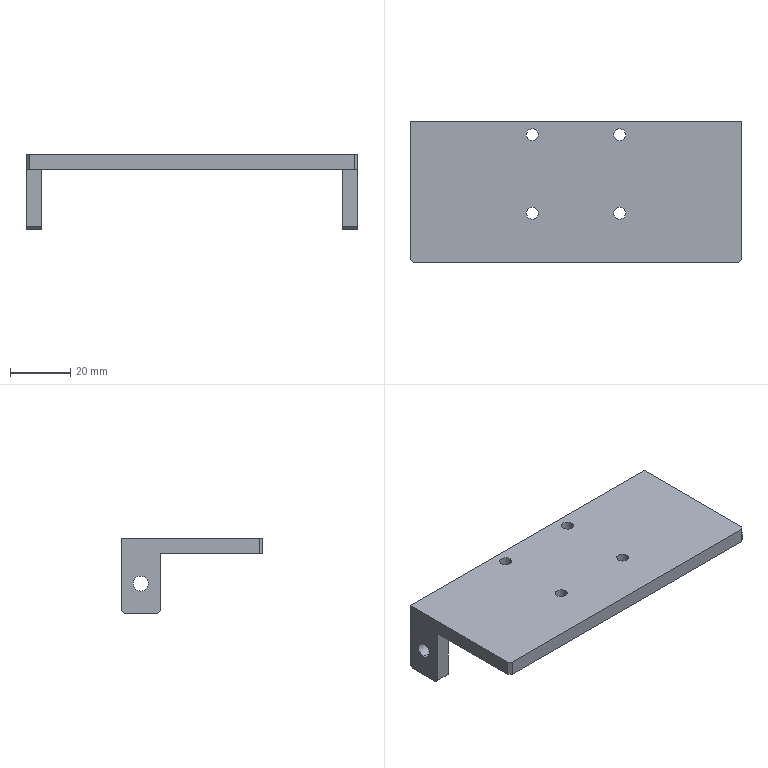Part | STEP file | Guide wheel mechanism revised.sldasm-Part-392 | 1 solid | 30 faces | box 110 x 47 x 25 mm | volume 27987 mm3 | plane 18 | cylinder 12 | commonest cylinder face diameters 4 x8 5 x4
STEP:
#1=CARTESIAN_POINT('',(55.,40.5,-12.5));
#2=VERTEX_POINT('',#1);
#3=CARTESIAN_POINT('',(55.,40.5,-17.5));
#4=VERTEX_POINT('',#3);
#5=CARTESIAN_POINT('',(55.,40.5,-15.));
#6=DIRECTION('',(1.,0.,0.));
#7=DIRECTION('',(0.,0.,1.));
#8=AXIS2_PLACEMENT_3D('',#5,#6,#7);
#9=CIRCLE('',#8,2.5);
#10=EDGE_CURVE('',#2,#4,#9,.T.);
#11=ORIENTED_EDGE('',*,*,#10,.T.);
#12=CARTESIAN_POINT('',(50.,40.5,-17.5));
#13=VERTEX_POINT('',#12);
#14=CARTESIAN_POINT('',(94.446,40.5,-17.5));
#15=DIRECTION('',(-1.,0.,0.));
#16=VECTOR('',#15,1000.);
#17=LINE('',#14,#16);
#18=EDGE_CURVE('',#4,#13,#17,.T.);
#19=ORIENTED_EDGE('',*,*,#18,.T.);
#20=CARTESIAN_POINT('',(50.,40.5,-12.5));
#21=VERTEX_POINT('',#20);
#22=CARTESIAN_POINT('',(50.,40.5,-15.));
#23=DIRECTION('',(-1.,0.,0.));
#24=DIRECTION('',(0.,0.,1.));
#25=AXIS2_PLACEMENT_3D('',#22,#23,#24);
#26=CIRCLE('',#25,2.5);
#27=EDGE_CURVE('',#13,#21,#26,.T.);
#28=ORIENTED_EDGE('',*,*,#27,.T.);
#29=CARTESIAN_POINT('',(94.446,40.5,-12.5));
#30=DIRECTION('',(-1.,0.,0.));
#31=VECTOR('',#30,1000.);
#32=LINE('',#29,#31);
#33=EDGE_CURVE('',#2,#21,#32,.T.);
#34=ORIENTED_EDGE('',*,*,#33,.F.);
#35=EDGE_LOOP('',(#11,#19,#28,#34));
#36=FACE_OUTER_BOUND('',#35,.T.);
#37=CARTESIAN_POINT('',(94.446,40.5,-15.));
#38=DIRECTION('',(-1.,0.,0.));
#39=DIRECTION('',(0.,0.,1.));
#40=AXIS2_PLACEMENT_3D('',#37,#38,#39);
#41=CYLINDRICAL_SURFACE('',#40,2.5);
#42=ADVANCED_FACE('',(#36),#41,.F.);
#43=CARTESIAN_POINT('',(-50.,40.5,-12.5));
#44=VERTEX_POINT('',#43);
#45=CARTESIAN_POINT('',(-50.,40.5,-17.5));
#46=VERTEX_POINT('',#45);
#47=CARTESIAN_POINT('',(-50.,40.5,-15.));
#48=DIRECTION('',(1.,0.,0.));
#49=DIRECTION('',(0.,0.,-1.));
#50=AXIS2_PLACEMENT_3D('',#47,#48,#49);
#51=CIRCLE('',#50,2.5);
#52=EDGE_CURVE('',#44,#46,#51,.T.);
#53=ORIENTED_EDGE('',*,*,#52,.T.);
#54=CARTESIAN_POINT('',(-55.,40.5,-17.5));
#55=VERTEX_POINT('',#54);
#56=CARTESIAN_POINT('',(94.446,40.5,-17.5));
#57=DIRECTION('',(-1.,0.,0.));
#58=VECTOR('',#57,1000.);
#59=LINE('',#56,#58);
#60=EDGE_CURVE('',#46,#55,#59,.T.);
#61=ORIENTED_EDGE('',*,*,#60,.T.);
#62=CARTESIAN_POINT('',(-55.,40.5,-12.5));
#63=VERTEX_POINT('',#62);
#64=CARTESIAN_POINT('',(-55.,40.5,-15.));
#65=DIRECTION('',(-1.,0.,0.));
#66=DIRECTION('',(0.,0.,1.));
#67=AXIS2_PLACEMENT_3D('',#64,#65,#66);
#68=CIRCLE('',#67,2.5);
#69=EDGE_CURVE('',#55,#63,#68,.T.);
#70=ORIENTED_EDGE('',*,*,#69,.T.);
#71=CARTESIAN_POINT('',(94.446,40.5,-12.5));
#72=DIRECTION('',(-1.,0.,0.));
#73=VECTOR('',#72,1000.);
#74=LINE('',#71,#73);
#75=EDGE_CURVE('',#44,#63,#74,.T.);
#76=ORIENTED_EDGE('',*,*,#75,.F.);
#77=EDGE_LOOP('',(#53,#61,#70,#76));
#78=FACE_OUTER_BOUND('',#77,.T.);
#79=CARTESIAN_POINT('',(94.446,40.5,-15.));
#80=DIRECTION('',(-1.,0.,0.));
#81=DIRECTION('',(0.,0.,1.));
#82=AXIS2_PLACEMENT_3D('',#79,#80,#81);
#83=CYLINDRICAL_SURFACE('',#82,2.5);
#84=ADVANCED_FACE('',(#78),#83,.F.);
#85=CARTESIAN_POINT('',(-16.5,16.5,-5.));
#86=VERTEX_POINT('',#85);
#87=CARTESIAN_POINT('',(-12.5,16.5,-5.));
#88=VERTEX_POINT('',#87);
#89=CARTESIAN_POINT('',(-14.5,16.5,-5.));
#90=DIRECTION('',(0.,0.,1.));
#91=DIRECTION('',(-1.,0.,0.));
#92=AXIS2_PLACEMENT_3D('',#89,#90,#91);
#93=CIRCLE('',#92,2.);
#94=EDGE_CURVE('',#86,#88,#93,.T.);
#95=ORIENTED_EDGE('',*,*,#94,.F.);
#96=CARTESIAN_POINT('',(-16.5,16.5,0.));
#97=VERTEX_POINT('',#96);
#98=CARTESIAN_POINT('',(-16.5,16.5,-25.001));
#99=DIRECTION('',(0.,0.,1.));
#100=VECTOR('',#99,1000.);
#101=LINE('',#98,#100);
#102=EDGE_CURVE('',#86,#97,#101,.T.);
#103=ORIENTED_EDGE('',*,*,#102,.T.);
#104=CARTESIAN_POINT('',(-12.5,16.5,0.));
#105=VERTEX_POINT('',#104);
#106=CARTESIAN_POINT('',(-14.5,16.5,0.));
#107=DIRECTION('',(0.,0.,1.));
#108=DIRECTION('',(1.,0.,0.));
#109=AXIS2_PLACEMENT_3D('',#106,#107,#108);
#110=CIRCLE('',#109,2.);
#111=EDGE_CURVE('',#97,#105,#110,.T.);
#112=ORIENTED_EDGE('',*,*,#111,.T.);
#113=CARTESIAN_POINT('',(-12.5,16.5,-25.001));
#114=DIRECTION('',(0.,0.,1.));
#115=VECTOR('',#114,1000.);
#116=LINE('',#113,#115);
#117=EDGE_CURVE('',#88,#105,#116,.T.);
#118=ORIENTED_EDGE('',*,*,#117,.F.);
#119=EDGE_LOOP('',(#95,#103,#112,#118));
#120=FACE_OUTER_BOUND('',#119,.T.);
#121=CARTESIAN_POINT('',(-14.5,16.5,-25.001));
#122=DIRECTION('',(0.,0.,1.));
#123=DIRECTION('',(1.,0.,0.));
#124=AXIS2_PLACEMENT_3D('',#121,#122,#123);
#125=CYLINDRICAL_SURFACE('',#124,2.);
#126=ADVANCED_FACE('',(#120),#125,.F.);
#127=CARTESIAN_POINT('',(12.5,16.5,-5.));
#128=VERTEX_POINT('',#127);
#129=CARTESIAN_POINT('',(16.5,16.5,-5.));
#130=VERTEX_POINT('',#129);
#131=CARTESIAN_POINT('',(14.5,16.5,-5.));
#132=DIRECTION('',(0.,0.,1.));
#133=DIRECTION('',(-1.,0.,0.));
#134=AXIS2_PLACEMENT_3D('',#131,#132,#133);
#135=CIRCLE('',#134,2.);
#136=EDGE_CURVE('',#128,#130,#135,.T.);
#137=ORIENTED_EDGE('',*,*,#136,.F.);
#138=CARTESIAN_POINT('',(12.5,16.5,0.));
#139=VERTEX_POINT('',#138);
#140=CARTESIAN_POINT('',(12.5,16.5,-25.001));
#141=DIRECTION('',(0.,0.,1.));
#142=VECTOR('',#141,1000.);
#143=LINE('',#140,#142);
#144=EDGE_CURVE('',#128,#139,#143,.T.);
#145=ORIENTED_EDGE('',*,*,#144,.T.);
#146=CARTESIAN_POINT('',(16.5,16.5,0.));
#147=VERTEX_POINT('',#146);
#148=CARTESIAN_POINT('',(14.5,16.5,0.));
#149=DIRECTION('',(0.,0.,1.));
#150=DIRECTION('',(1.,0.,0.));
#151=AXIS2_PLACEMENT_3D('',#148,#149,#150);
#152=CIRCLE('',#151,2.);
#153=EDGE_CURVE('',#139,#147,#152,.T.);
#154=ORIENTED_EDGE('',*,*,#153,.T.);
#155=CARTESIAN_POINT('',(16.5,16.5,-25.001));
#156=DIRECTION('',(0.,0.,1.));
#157=VECTOR('',#156,1000.);
#158=LINE('',#155,#157);
#159=EDGE_CURVE('',#130,#147,#158,.T.);
#160=ORIENTED_EDGE('',*,*,#159,.F.);
#161=EDGE_LOOP('',(#137,#145,#154,#160));
#162=FACE_OUTER_BOUND('',#161,.T.);
#163=CARTESIAN_POINT('',(14.5,16.5,-25.001));
#164=DIRECTION('',(0.,0.,1.));
#165=DIRECTION('',(1.,0.,0.));
#166=AXIS2_PLACEMENT_3D('',#163,#164,#165);
#167=CYLINDRICAL_SURFACE('',#166,2.);
#168=ADVANCED_FACE('',(#162),#167,.F.);
#169=CARTESIAN_POINT('',(12.5,42.5,-5.));
#170=VERTEX_POINT('',#169);
#171=CARTESIAN_POINT('',(16.5,42.5,-5.));
#172=VERTEX_POINT('',#171);
#173=CARTESIAN_POINT('',(14.5,42.5,-5.));
#174=DIRECTION('',(0.,0.,1.));
#175=DIRECTION('',(-1.,0.,0.));
#176=AXIS2_PLACEMENT_3D('',#173,#174,#175);
#177=CIRCLE('',#176,2.);
#178=EDGE_CURVE('',#170,#172,#177,.T.);
#179=ORIENTED_EDGE('',*,*,#178,.F.);
#180=CARTESIAN_POINT('',(12.5,42.5,0.));
#181=VERTEX_POINT('',#180);
#182=CARTESIAN_POINT('',(12.5,42.5,-25.001));
#183=DIRECTION('',(0.,0.,1.));
#184=VECTOR('',#183,1000.);
#185=LINE('',#182,#184);
#186=EDGE_CURVE('',#170,#181,#185,.T.);
#187=ORIENTED_EDGE('',*,*,#186,.T.);
#188=CARTESIAN_POINT('',(16.5,42.5,0.));
#189=VERTEX_POINT('',#188);
#190=CARTESIAN_POINT('',(14.5,42.5,0.));
#191=DIRECTION('',(0.,0.,1.));
#192=DIRECTION('',(1.,0.,0.));
#193=AXIS2_PLACEMENT_3D('',#190,#191,#192);
#194=CIRCLE('',#193,2.);
#195=EDGE_CURVE('',#181,#189,#194,.T.);
#196=ORIENTED_EDGE('',*,*,#195,.T.);
#197=CARTESIAN_POINT('',(16.5,42.5,-25.001));
#198=DIRECTION('',(0.,0.,1.));
#199=VECTOR('',#198,1000.);
#200=LINE('',#197,#199);
#201=EDGE_CURVE('',#172,#189,#200,.T.);
#202=ORIENTED_EDGE('',*,*,#201,.F.);
#203=EDGE_LOOP('',(#179,#187,#196,#202));
#204=FACE_OUTER_BOUND('',#203,.T.);
#205=CARTESIAN_POINT('',(14.5,42.5,-25.001));
#206=DIRECTION('',(0.,0.,1.));
#207=DIRECTION('',(1.,0.,0.));
#208=AXIS2_PLACEMENT_3D('',#205,#206,#207);
#209=CYLINDRICAL_SURFACE('',#208,2.);
#210=ADVANCED_FACE('',(#204),#209,.F.);
#211=CARTESIAN_POINT('',(-16.5,42.5,-5.));
#212=VERTEX_POINT('',#211);
#213=CARTESIAN_POINT('',(-12.5,42.5,-5.));
#214=VERTEX_POINT('',#213);
#215=CARTESIAN_POINT('',(-14.5,42.5,-5.));
#216=DIRECTION('',(0.,0.,1.));
#217=DIRECTION('',(-1.,0.,0.));
#218=AXIS2_PLACEMENT_3D('',#215,#216,#217);
#219=CIRCLE('',#218,2.);
#220=EDGE_CURVE('',#212,#214,#219,.T.);
#221=ORIENTED_EDGE('',*,*,#220,.F.);
#222=CARTESIAN_POINT('',(-16.5,42.5,0.));
#223=VERTEX_POINT('',#222);
#224=CARTESIAN_POINT('',(-16.5,42.5,-25.001));
#225=DIRECTION('',(0.,0.,1.));
#226=VECTOR('',#225,1000.);
#227=LINE('',#224,#226);
#228=EDGE_CURVE('',#212,#223,#227,.T.);
#229=ORIENTED_EDGE('',*,*,#228,.T.);
#230=CARTESIAN_POINT('',(-12.5,42.5,0.));
#231=VERTEX_POINT('',#230);
#232=CARTESIAN_POINT('',(-14.5,42.5,0.));
#233=DIRECTION('',(0.,0.,1.));
#234=DIRECTION('',(1.,0.,0.));
#235=AXIS2_PLACEMENT_3D('',#232,#233,#234);
#236=CIRCLE('',#235,2.);
#237=EDGE_CURVE('',#223,#231,#236,.T.);
#238=ORIENTED_EDGE('',*,*,#237,.T.);
#239=CARTESIAN_POINT('',(-12.5,42.5,-25.001));
#240=DIRECTION('',(0.,0.,1.));
#241=VECTOR('',#240,1000.);
#242=LINE('',#239,#241);
#243=EDGE_CURVE('',#214,#231,#242,.T.);
#244=ORIENTED_EDGE('',*,*,#243,.F.);
#245=EDGE_LOOP('',(#221,#229,#238,#244));
#246=FACE_OUTER_BOUND('',#245,.T.);
#247=CARTESIAN_POINT('',(-14.5,42.5,-25.001));
#248=DIRECTION('',(0.,0.,1.));
#249=DIRECTION('',(1.,0.,0.));
#250=AXIS2_PLACEMENT_3D('',#247,#248,#249);
#251=CYLINDRICAL_SURFACE('',#250,2.);
#252=ADVANCED_FACE('',(#246),#251,.F.);
#253=ORIENTED_EDGE('',*,*,#10,.F.);
#254=CARTESIAN_POINT('',(55.,40.5,-15.));
#255=DIRECTION('',(1.,0.,0.));
#256=DIRECTION('',(0.,0.,1.));
#257=AXIS2_PLACEMENT_3D('',#254,#255,#256);
#258=CIRCLE('',#257,2.5);
#259=EDGE_CURVE('',#4,#2,#258,.T.);
#260=ORIENTED_EDGE('',*,*,#259,.F.);
#261=EDGE_LOOP('',(#253,#260));
#262=FACE_BOUND('',#261,.T.);
#263=CARTESIAN_POINT('',(55.,47.,0.));
#264=VERTEX_POINT('',#263);
#265=CARTESIAN_POINT('',(55.,1.,0.));
#266=VERTEX_POINT('',#265);
#267=CARTESIAN_POINT('',(55.,47.,0.));
#268=DIRECTION('',(0.,-1.,0.));
#269=VECTOR('',#268,1000.);
#270=LINE('',#267,#269);
#271=EDGE_CURVE('',#264,#266,#270,.T.);
#272=ORIENTED_EDGE('',*,*,#271,.T.);
#273=CARTESIAN_POINT('',(55.,1.,-5.));
#274=VERTEX_POINT('',#273);
#275=CARTESIAN_POINT('',(55.,1.,-5.));
#276=DIRECTION('',(0.,0.,-1.));
#277=VECTOR('',#276,1000.);
#278=LINE('',#275,#277);
#279=EDGE_CURVE('',#266,#274,#278,.T.);
#280=ORIENTED_EDGE('',*,*,#279,.T.);
#281=CARTESIAN_POINT('',(55.,34.,-5.));
#282=VERTEX_POINT('',#281);
#283=CARTESIAN_POINT('',(55.,0.,-5.));
#284=DIRECTION('',(0.,-1.,0.));
#285=VECTOR('',#284,1000.);
#286=LINE('',#283,#285);
#287=EDGE_CURVE('',#282,#274,#286,.T.);
#288=ORIENTED_EDGE('',*,*,#287,.F.);
#289=CARTESIAN_POINT('',(55.,34.,-24.));
#290=VERTEX_POINT('',#289);
#291=CARTESIAN_POINT('',(55.,34.,-25.));
#292=DIRECTION('',(0.,0.,1.));
#293=VECTOR('',#292,1000.);
#294=LINE('',#291,#293);
#295=EDGE_CURVE('',#290,#282,#294,.T.);
#296=ORIENTED_EDGE('',*,*,#295,.F.);
#297=CARTESIAN_POINT('',(55.,35.,-25.));
#298=VERTEX_POINT('',#297);
#299=CARTESIAN_POINT('',(55.,35.,-25.));
#300=DIRECTION('',(0.,0.7071,-0.7071));
#301=VECTOR('',#300,1000.);
#302=LINE('',#299,#301);
#303=EDGE_CURVE('',#290,#298,#302,.T.);
#304=ORIENTED_EDGE('',*,*,#303,.T.);
#305=CARTESIAN_POINT('',(55.,46.,-25.));
#306=VERTEX_POINT('',#305);
#307=CARTESIAN_POINT('',(55.,47.,-25.));
#308=DIRECTION('',(0.,-1.,0.));
#309=VECTOR('',#308,1000.);
#310=LINE('',#307,#309);
#311=EDGE_CURVE('',#306,#298,#310,.T.);
#312=ORIENTED_EDGE('',*,*,#311,.F.);
#313=CARTESIAN_POINT('',(55.,47.,-24.));
#314=VERTEX_POINT('',#313);
#315=CARTESIAN_POINT('',(55.,46.,-25.));
#316=DIRECTION('',(0.,0.7071,0.7071));
#317=VECTOR('',#316,1000.);
#318=LINE('',#315,#317);
#319=EDGE_CURVE('',#306,#314,#318,.T.);
#320=ORIENTED_EDGE('',*,*,#319,.T.);
#321=CARTESIAN_POINT('',(55.,47.,0.));
#322=DIRECTION('',(0.,0.,-1.));
#323=VECTOR('',#322,1000.);
#324=LINE('',#321,#323);
#325=EDGE_CURVE('',#264,#314,#324,.T.);
#326=ORIENTED_EDGE('',*,*,#325,.F.);
#327=EDGE_LOOP('',(#272,#280,#288,#296,#304,#312,#320,#326));
#328=FACE_OUTER_BOUND('',#327,.T.);
#329=CARTESIAN_POINT('',(55.,47.,0.));
#330=DIRECTION('',(-1.,0.,0.));
#331=DIRECTION('',(0.,0.,1.));
#332=AXIS2_PLACEMENT_3D('',#329,#330,#331);
#333=PLANE('',#332);
#334=ADVANCED_FACE('',(#262,#328),#333,.F.);
#335=ORIENTED_EDGE('',*,*,#311,.T.);
#336=CARTESIAN_POINT('',(50.,35.,-25.));
#337=VERTEX_POINT('',#336);
#338=CARTESIAN_POINT('',(50.,35.,-25.));
#339=DIRECTION('',(-1.,0.,0.));
#340=VECTOR('',#339,1000.);
#341=LINE('',#338,#340);
#342=EDGE_CURVE('',#298,#337,#341,.T.);
#343=ORIENTED_EDGE('',*,*,#342,.T.);
#344=CARTESIAN_POINT('',(50.,46.,-25.));
#345=VERTEX_POINT('',#344);
#346=CARTESIAN_POINT('',(50.,47.,-25.));
#347=DIRECTION('',(0.,-1.,0.));
#348=VECTOR('',#347,1000.);
#349=LINE('',#346,#348);
#350=EDGE_CURVE('',#345,#337,#349,.T.);
#351=ORIENTED_EDGE('',*,*,#350,.F.);
#352=CARTESIAN_POINT('',(55.,46.,-25.));
#353=DIRECTION('',(1.,0.,0.));
#354=VECTOR('',#353,1000.);
#355=LINE('',#352,#354);
#356=EDGE_CURVE('',#345,#306,#355,.T.);
#357=ORIENTED_EDGE('',*,*,#356,.T.);
#358=EDGE_LOOP('',(#335,#343,#351,#357));
#359=FACE_OUTER_BOUND('',#358,.T.);
#360=CARTESIAN_POINT('',(50.,47.,-25.));
#361=DIRECTION('',(0.,0.,-1.));
#362=DIRECTION('',(-1.,0.,0.));
#363=AXIS2_PLACEMENT_3D('',#360,#361,#362);
#364=PLANE('',#363);
#365=ADVANCED_FACE('',(#359),#364,.T.);
#366=CARTESIAN_POINT('',(50.,40.5,-15.));
#367=DIRECTION('',(-1.,0.,0.));
#368=DIRECTION('',(0.,0.,1.));
#369=AXIS2_PLACEMENT_3D('',#366,#367,#368);
#370=CIRCLE('',#369,2.5);
#371=EDGE_CURVE('',#21,#13,#370,.T.);
#372=ORIENTED_EDGE('',*,*,#371,.F.);
#373=ORIENTED_EDGE('',*,*,#27,.F.);
#374=EDGE_LOOP('',(#372,#373));
#375=FACE_BOUND('',#374,.T.);
#376=ORIENTED_EDGE('',*,*,#350,.T.);
#377=CARTESIAN_POINT('',(50.,34.,-24.));
#378=VERTEX_POINT('',#377);
#379=CARTESIAN_POINT('',(50.,28.5,-18.5));
#380=DIRECTION('',(0.,-0.7071,0.7071));
#381=VECTOR('',#380,1000.);
#382=LINE('',#379,#381);
#383=EDGE_CURVE('',#337,#378,#382,.T.);
#384=ORIENTED_EDGE('',*,*,#383,.T.);
#385=CARTESIAN_POINT('',(50.,34.,-5.));
#386=VERTEX_POINT('',#385);
#387=CARTESIAN_POINT('',(50.,34.,0.));
#388=DIRECTION('',(0.,0.,-1.));
#389=VECTOR('',#388,1000.);
#390=LINE('',#387,#389);
#391=EDGE_CURVE('',#386,#378,#390,.T.);
#392=ORIENTED_EDGE('',*,*,#391,.F.);
#393=CARTESIAN_POINT('',(50.,47.,-5.));
#394=VERTEX_POINT('',#393);
#395=CARTESIAN_POINT('',(50.,47.,-5.));
#396=DIRECTION('',(0.,-1.,0.));
#397=VECTOR('',#396,1000.);
#398=LINE('',#395,#397);
#399=EDGE_CURVE('',#394,#386,#398,.T.);
#400=ORIENTED_EDGE('',*,*,#399,.F.);
#401=CARTESIAN_POINT('',(50.,47.,-24.));
#402=VERTEX_POINT('',#401);
#403=CARTESIAN_POINT('',(50.,47.,0.));
#404=DIRECTION('',(0.,0.,-1.));
#405=VECTOR('',#404,1000.);
#406=LINE('',#403,#405);
#407=EDGE_CURVE('',#394,#402,#406,.T.);
#408=ORIENTED_EDGE('',*,*,#407,.T.);
#409=CARTESIAN_POINT('',(50.,59.,-12.));
#410=DIRECTION('',(0.,-0.7071,-0.7071));
#411=VECTOR('',#410,1000.);
#412=LINE('',#409,#411);
#413=EDGE_CURVE('',#402,#345,#412,.T.);
#414=ORIENTED_EDGE('',*,*,#413,.T.);
#415=EDGE_LOOP('',(#376,#384,#392,#400,#408,#414));
#416=FACE_OUTER_BOUND('',#415,.T.);
#417=CARTESIAN_POINT('',(50.,47.,0.));
#418=DIRECTION('',(-1.,0.,0.));
#419=DIRECTION('',(0.,0.,1.));
#420=AXIS2_PLACEMENT_3D('',#417,#418,#419);
#421=PLANE('',#420);
#422=ADVANCED_FACE('',(#375,#416),#421,.T.);
#423=ORIENTED_EDGE('',*,*,#287,.T.);
#424=CARTESIAN_POINT('',(54.,0.,-5.));
#425=VERTEX_POINT('',#424);
#426=CARTESIAN_POINT('',(23.,-31.,-5.));
#427=DIRECTION('',(-0.7071,-0.7071,0.));
#428=VECTOR('',#427,1000.);
#429=LINE('',#426,#428);
#430=EDGE_CURVE('',#274,#425,#429,.T.);
#431=ORIENTED_EDGE('',*,*,#430,.T.);
#432=CARTESIAN_POINT('',(-54.,0.,-5.));
#433=VERTEX_POINT('',#432);
#434=CARTESIAN_POINT('',(-55.,0.,-5.));
#435=DIRECTION('',(1.,0.,0.));
#436=VECTOR('',#435,1000.);
#437=LINE('',#434,#436);
#438=EDGE_CURVE('',#433,#425,#437,.T.);
#439=ORIENTED_EDGE('',*,*,#438,.F.);
#440=CARTESIAN_POINT('',(-55.,1.,-5.));
#441=VERTEX_POINT('',#440);
#442=CARTESIAN_POINT('',(-78.,24.,-5.));
#443=DIRECTION('',(-0.7071,0.7071,0.));
#444=VECTOR('',#443,1000.);
#445=LINE('',#442,#444);
#446=EDGE_CURVE('',#433,#441,#445,.T.);
#447=ORIENTED_EDGE('',*,*,#446,.T.);
#448=CARTESIAN_POINT('',(-55.,34.,-5.));
#449=VERTEX_POINT('',#448);
#450=CARTESIAN_POINT('',(-55.,0.,-5.));
#451=DIRECTION('',(0.,1.,0.));
#452=VECTOR('',#451,1000.);
#453=LINE('',#450,#452);
#454=EDGE_CURVE('',#441,#449,#453,.T.);
#455=ORIENTED_EDGE('',*,*,#454,.T.);
#456=CARTESIAN_POINT('',(-50.,34.,-5.));
#457=VERTEX_POINT('',#456);
#458=CARTESIAN_POINT('',(94.446,34.,-5.));
#459=DIRECTION('',(-1.,0.,0.));
#460=VECTOR('',#459,1000.);
#461=LINE('',#458,#460);
#462=EDGE_CURVE('',#457,#449,#461,.T.);
#463=ORIENTED_EDGE('',*,*,#462,.F.);
#464=CARTESIAN_POINT('',(-50.,47.,-5.));
#465=VERTEX_POINT('',#464);
#466=CARTESIAN_POINT('',(-50.,47.,-5.));
#467=DIRECTION('',(0.,-1.,0.));
#468=VECTOR('',#467,1000.);
#469=LINE('',#466,#468);
#470=EDGE_CURVE('',#465,#457,#469,.T.);
#471=ORIENTED_EDGE('',*,*,#470,.F.);
#472=CARTESIAN_POINT('',(-55.,47.,-5.));
#473=DIRECTION('',(1.,0.,0.));
#474=VECTOR('',#473,1000.);
#475=LINE('',#472,#474);
#476=EDGE_CURVE('',#465,#394,#475,.T.);
#477=ORIENTED_EDGE('',*,*,#476,.T.);
#478=ORIENTED_EDGE('',*,*,#399,.T.);
#479=CARTESIAN_POINT('',(94.446,34.,-5.));
#480=DIRECTION('',(-1.,0.,0.));
#481=VECTOR('',#480,1000.);
#482=LINE('',#479,#481);
#483=EDGE_CURVE('',#282,#386,#482,.T.);
#484=ORIENTED_EDGE('',*,*,#483,.F.);
#485=EDGE_LOOP('',(#423,#431,#439,#447,#455,#463,#471,#477,#478,#484));
#486=FACE_OUTER_BOUND('',#485,.T.);
#487=CARTESIAN_POINT('',(14.5,42.5,-5.));
#488=DIRECTION('',(0.,0.,1.));
#489=DIRECTION('',(-1.,0.,0.));
#490=AXIS2_PLACEMENT_3D('',#487,#488,#489);
#491=CIRCLE('',#490,2.);
#492=EDGE_CURVE('',#172,#170,#491,.T.);
#493=ORIENTED_EDGE('',*,*,#492,.T.);
#494=ORIENTED_EDGE('',*,*,#178,.T.);
#495=EDGE_LOOP('',(#493,#494));
#496=FACE_BOUND('',#495,.T.);
#497=CARTESIAN_POINT('',(-14.5,42.5,-5.));
#498=DIRECTION('',(0.,0.,1.));
#499=DIRECTION('',(-1.,0.,0.));
#500=AXIS2_PLACEMENT_3D('',#497,#498,#499);
#501=CIRCLE('',#500,2.);
#502=EDGE_CURVE('',#214,#212,#501,.T.);
#503=ORIENTED_EDGE('',*,*,#502,.T.);
#504=ORIENTED_EDGE('',*,*,#220,.T.);
#505=EDGE_LOOP('',(#503,#504));
#506=FACE_BOUND('',#505,.T.);
#507=CARTESIAN_POINT('',(14.5,16.5,-5.));
#508=DIRECTION('',(0.,0.,1.));
#509=DIRECTION('',(-1.,0.,0.));
#510=AXIS2_PLACEMENT_3D('',#507,#508,#509);
#511=CIRCLE('',#510,2.);
#512=EDGE_CURVE('',#130,#128,#511,.T.);
#513=ORIENTED_EDGE('',*,*,#512,.T.);
#514=ORIENTED_EDGE('',*,*,#136,.T.);
#515=EDGE_LOOP('',(#513,#514));
#516=FACE_BOUND('',#515,.T.);
#517=CARTESIAN_POINT('',(-14.5,16.5,-5.));
#518=DIRECTION('',(0.,0.,1.));
#519=DIRECTION('',(-1.,0.,0.));
#520=AXIS2_PLACEMENT_3D('',#517,#518,#519);
#521=CIRCLE('',#520,2.);
#522=EDGE_CURVE('',#88,#86,#521,.T.);
#523=ORIENTED_EDGE('',*,*,#522,.T.);
#524=ORIENTED_EDGE('',*,*,#94,.T.);
#525=EDGE_LOOP('',(#523,#524));
#526=FACE_BOUND('',#525,.T.);
#527=CARTESIAN_POINT('',(-55.,47.,-5.));
#528=DIRECTION('',(0.,0.,-1.));
#529=DIRECTION('',(-1.,0.,0.));
#530=AXIS2_PLACEMENT_3D('',#527,#528,#529);
#531=PLANE('',#530);
#532=ADVANCED_FACE('',(#486,#496,#506,#516,#526),#531,.T.);
#533=ORIENTED_EDGE('',*,*,#52,.F.);
#534=CARTESIAN_POINT('',(-50.,40.5,-15.));
#535=DIRECTION('',(1.,0.,0.));
#536=DIRECTION('',(0.,0.,-1.));
#537=AXIS2_PLACEMENT_3D('',#534,#535,#536);
#538=CIRCLE('',#537,2.5);
#539=EDGE_CURVE('',#46,#44,#538,.T.);
#540=ORIENTED_EDGE('',*,*,#539,.F.);
#541=EDGE_LOOP('',(#533,#540));
#542=FACE_BOUND('',#541,.T.);
#543=CARTESIAN_POINT('',(-50.,34.,-24.));
#544=VERTEX_POINT('',#543);
#545=CARTESIAN_POINT('',(-50.,34.,-25.));
#546=DIRECTION('',(0.,0.,1.));
#547=VECTOR('',#546,1000.);
#548=LINE('',#545,#547);
#549=EDGE_CURVE('',#544,#457,#548,.T.);
#550=ORIENTED_EDGE('',*,*,#549,.F.);
#551=CARTESIAN_POINT('',(-50.,35.,-25.));
#552=VERTEX_POINT('',#551);
#553=CARTESIAN_POINT('',(-50.,41.,-31.));
#554=DIRECTION('',(0.,0.7071,-0.7071));
#555=VECTOR('',#554,1000.);
#556=LINE('',#553,#555);
#557=EDGE_CURVE('',#544,#552,#556,.T.);
#558=ORIENTED_EDGE('',*,*,#557,.T.);
#559=CARTESIAN_POINT('',(-50.,46.,-25.));
#560=VERTEX_POINT('',#559);
#561=CARTESIAN_POINT('',(-50.,47.,-25.));
#562=DIRECTION('',(0.,-1.,0.));
#563=VECTOR('',#562,1000.);
#564=LINE('',#561,#563);
#565=EDGE_CURVE('',#560,#552,#564,.T.);
#566=ORIENTED_EDGE('',*,*,#565,.F.);
#567=CARTESIAN_POINT('',(-50.,47.,-24.));
#568=VERTEX_POINT('',#567);
#569=CARTESIAN_POINT('',(-50.,46.5,-24.5));
#570=DIRECTION('',(0.,0.7071,0.7071));
#571=VECTOR('',#570,1000.);
#572=LINE('',#569,#571);
#573=EDGE_CURVE('',#560,#568,#572,.T.);
#574=ORIENTED_EDGE('',*,*,#573,.T.);
#575=CARTESIAN_POINT('',(-50.,47.,-25.));
#576=DIRECTION('',(0.,0.,1.));
#577=VECTOR('',#576,1000.);
#578=LINE('',#575,#577);
#579=EDGE_CURVE('',#568,#465,#578,.T.);
#580=ORIENTED_EDGE('',*,*,#579,.T.);
#581=ORIENTED_EDGE('',*,*,#470,.T.);
#582=EDGE_LOOP('',(#550,#558,#566,#574,#580,#581));
#583=FACE_OUTER_BOUND('',#582,.T.);
#584=CARTESIAN_POINT('',(-50.,47.,-25.));
#585=DIRECTION('',(1.,0.,0.));
#586=DIRECTION('',(0.,0.,-1.));
#587=AXIS2_PLACEMENT_3D('',#584,#585,#586);
#588=PLANE('',#587);
#589=ADVANCED_FACE('',(#542,#583),#588,.T.);
#590=ORIENTED_EDGE('',*,*,#565,.T.);
#591=CARTESIAN_POINT('',(-55.,35.,-25.));
#592=VERTEX_POINT('',#591);
#593=CARTESIAN_POINT('',(-55.,35.,-25.));
#594=DIRECTION('',(-1.,0.,0.));
#595=VECTOR('',#594,1000.);
#596=LINE('',#593,#595);
#597=EDGE_CURVE('',#552,#592,#596,.T.);
#598=ORIENTED_EDGE('',*,*,#597,.T.);
#599=CARTESIAN_POINT('',(-55.,46.,-25.));
#600=VERTEX_POINT('',#599);
#601=CARTESIAN_POINT('',(-55.,47.,-25.));
#602=DIRECTION('',(0.,-1.,0.));
#603=VECTOR('',#602,1000.);
#604=LINE('',#601,#603);
#605=EDGE_CURVE('',#600,#592,#604,.T.);
#606=ORIENTED_EDGE('',*,*,#605,.F.);
#607=CARTESIAN_POINT('',(-50.,46.,-25.));
#608=DIRECTION('',(1.,0.,0.));
#609=VECTOR('',#608,1000.);
#610=LINE('',#607,#609);
#611=EDGE_CURVE('',#600,#560,#610,.T.);
#612=ORIENTED_EDGE('',*,*,#611,.T.);
#613=EDGE_LOOP('',(#590,#598,#606,#612));
#614=FACE_OUTER_BOUND('',#613,.T.);
#615=CARTESIAN_POINT('',(-55.,47.,-25.));
#616=DIRECTION('',(0.,0.,-1.));
#617=DIRECTION('',(-1.,0.,0.));
#618=AXIS2_PLACEMENT_3D('',#615,#616,#617);
#619=PLANE('',#618);
#620=ADVANCED_FACE('',(#614),#619,.T.);
#621=CARTESIAN_POINT('',(-55.,40.5,-15.));
#622=DIRECTION('',(-1.,0.,0.));
#623=DIRECTION('',(0.,0.,1.));
#624=AXIS2_PLACEMENT_3D('',#621,#622,#623);
#625=CIRCLE('',#624,2.5);
#626=EDGE_CURVE('',#63,#55,#625,.T.);
#627=ORIENTED_EDGE('',*,*,#626,.F.);
#628=ORIENTED_EDGE('',*,*,#69,.F.);
#629=EDGE_LOOP('',(#627,#628));
#630=FACE_BOUND('',#629,.T.);
#631=ORIENTED_EDGE('',*,*,#454,.F.);
#632=CARTESIAN_POINT('',(-55.,1.,0.));
#633=VERTEX_POINT('',#632);
#634=CARTESIAN_POINT('',(-55.,1.,0.));
#635=DIRECTION('',(0.,0.,1.));
#636=VECTOR('',#635,1000.);
#637=LINE('',#634,#636);
#638=EDGE_CURVE('',#441,#633,#637,.T.);
#639=ORIENTED_EDGE('',*,*,#638,.T.);
#640=CARTESIAN_POINT('',(-55.,47.,0.));
#641=VERTEX_POINT('',#640);
#642=CARTESIAN_POINT('',(-55.,47.,0.));
#643=DIRECTION('',(0.,-1.,0.));
#644=VECTOR('',#643,1000.);
#645=LINE('',#642,#644);
#646=EDGE_CURVE('',#641,#633,#645,.T.);
#647=ORIENTED_EDGE('',*,*,#646,.F.);
#648=CARTESIAN_POINT('',(-55.,47.,-24.));
#649=VERTEX_POINT('',#648);
#650=CARTESIAN_POINT('',(-55.,47.,-25.));
#651=DIRECTION('',(0.,0.,1.));
#652=VECTOR('',#651,1000.);
#653=LINE('',#650,#652);
#654=EDGE_CURVE('',#649,#641,#653,.T.);
#655=ORIENTED_EDGE('',*,*,#654,.F.);
#656=CARTESIAN_POINT('',(-55.,46.,-25.));
#657=DIRECTION('',(0.,-0.7071,-0.7071));
#658=VECTOR('',#657,1000.);
#659=LINE('',#656,#658);
#660=EDGE_CURVE('',#649,#600,#659,.T.);
#661=ORIENTED_EDGE('',*,*,#660,.T.);
#662=ORIENTED_EDGE('',*,*,#605,.T.);
#663=CARTESIAN_POINT('',(-55.,34.,-24.));
#664=VERTEX_POINT('',#663);
#665=CARTESIAN_POINT('',(-55.,35.,-25.));
#666=DIRECTION('',(0.,-0.7071,0.7071));
#667=VECTOR('',#666,1000.);
#668=LINE('',#665,#667);
#669=EDGE_CURVE('',#592,#664,#668,.T.);
#670=ORIENTED_EDGE('',*,*,#669,.T.);
#671=CARTESIAN_POINT('',(-55.,34.,-25.));
#672=DIRECTION('',(0.,0.,-1.));
#673=VECTOR('',#672,1000.);
#674=LINE('',#671,#673);
#675=EDGE_CURVE('',#449,#664,#674,.T.);
#676=ORIENTED_EDGE('',*,*,#675,.F.);
#677=EDGE_LOOP('',(#631,#639,#647,#655,#661,#662,#670,#676));
#678=FACE_OUTER_BOUND('',#677,.T.);
#679=CARTESIAN_POINT('',(-55.,47.,-25.));
#680=DIRECTION('',(1.,0.,0.));
#681=DIRECTION('',(0.,0.,-1.));
#682=AXIS2_PLACEMENT_3D('',#679,#680,#681);
#683=PLANE('',#682);
#684=ADVANCED_FACE('',(#630,#678),#683,.F.);
#685=CARTESIAN_POINT('',(-14.5,16.5,0.));
#686=DIRECTION('',(0.,0.,1.));
#687=DIRECTION('',(1.,0.,0.));
#688=AXIS2_PLACEMENT_3D('',#685,#686,#687);
#689=CIRCLE('',#688,2.);
#690=EDGE_CURVE('',#105,#97,#689,.T.);
#691=ORIENTED_EDGE('',*,*,#690,.F.);
#692=ORIENTED_EDGE('',*,*,#111,.F.);
#693=EDGE_LOOP('',(#691,#692));
#694=FACE_BOUND('',#693,.T.);
#695=CARTESIAN_POINT('',(14.5,16.5,0.));
#696=DIRECTION('',(0.,0.,1.));
#697=DIRECTION('',(1.,0.,0.));
#698=AXIS2_PLACEMENT_3D('',#695,#696,#697);
#699=CIRCLE('',#698,2.);
#700=EDGE_CURVE('',#147,#139,#699,.T.);
#701=ORIENTED_EDGE('',*,*,#700,.F.);
#702=ORIENTED_EDGE('',*,*,#153,.F.);
#703=EDGE_LOOP('',(#701,#702));
#704=FACE_BOUND('',#703,.T.);
#705=CARTESIAN_POINT('',(14.5,42.5,0.));
#706=DIRECTION('',(0.,0.,1.));
#707=DIRECTION('',(1.,0.,0.));
#708=AXIS2_PLACEMENT_3D('',#705,#706,#707);
#709=CIRCLE('',#708,2.);
#710=EDGE_CURVE('',#189,#181,#709,.T.);
#711=ORIENTED_EDGE('',*,*,#710,.F.);
#712=ORIENTED_EDGE('',*,*,#195,.F.);
#713=EDGE_LOOP('',(#711,#712));
#714=FACE_BOUND('',#713,.T.);
#715=CARTESIAN_POINT('',(-14.5,42.5,0.));
#716=DIRECTION('',(0.,0.,1.));
#717=DIRECTION('',(1.,0.,0.));
#718=AXIS2_PLACEMENT_3D('',#715,#716,#717);
#719=CIRCLE('',#718,2.);
#720=EDGE_CURVE('',#231,#223,#719,.T.);
#721=ORIENTED_EDGE('',*,*,#720,.F.);
#722=ORIENTED_EDGE('',*,*,#237,.F.);
#723=EDGE_LOOP('',(#721,#722));
#724=FACE_BOUND('',#723,.T.);
#725=CARTESIAN_POINT('',(-54.,0.,0.));
#726=VERTEX_POINT('',#725);
#727=CARTESIAN_POINT('',(54.,0.,0.));
#728=VERTEX_POINT('',#727);
#729=CARTESIAN_POINT('',(-55.,0.,0.));
#730=DIRECTION('',(1.,0.,0.));
#731=VECTOR('',#730,1000.);
#732=LINE('',#729,#731);
#733=EDGE_CURVE('',#726,#728,#732,.T.);
#734=ORIENTED_EDGE('',*,*,#733,.T.);
#735=CARTESIAN_POINT('',(55.,1.,0.));
#736=DIRECTION('',(0.7071,0.7071,0.));
#737=VECTOR('',#736,1000.);
#738=LINE('',#735,#737);
#739=EDGE_CURVE('',#728,#266,#738,.T.);
#740=ORIENTED_EDGE('',*,*,#739,.T.);
#741=ORIENTED_EDGE('',*,*,#271,.F.);
#742=CARTESIAN_POINT('',(-55.,47.,0.));
#743=DIRECTION('',(1.,0.,0.));
#744=VECTOR('',#743,1000.);
#745=LINE('',#742,#744);
#746=EDGE_CURVE('',#641,#264,#745,.T.);
#747=ORIENTED_EDGE('',*,*,#746,.F.);
#748=ORIENTED_EDGE('',*,*,#646,.T.);
#749=CARTESIAN_POINT('',(-55.,1.,0.));
#750=DIRECTION('',(0.7071,-0.7071,0.));
#751=VECTOR('',#750,1000.);
#752=LINE('',#749,#751);
#753=EDGE_CURVE('',#633,#726,#752,.T.);
#754=ORIENTED_EDGE('',*,*,#753,.T.);
#755=EDGE_LOOP('',(#734,#740,#741,#747,#748,#754));
#756=FACE_OUTER_BOUND('',#755,.T.);
#757=CARTESIAN_POINT('',(-55.,47.,0.));
#758=DIRECTION('',(0.,0.,-1.));
#759=DIRECTION('',(-1.,0.,0.));
#760=AXIS2_PLACEMENT_3D('',#757,#758,#759);
#761=PLANE('',#760);
#762=ADVANCED_FACE('',(#694,#704,#714,#724,#756),#761,.F.);
#763=ORIENTED_EDGE('',*,*,#579,.F.);
#764=CARTESIAN_POINT('',(-55.,47.,-24.));
#765=DIRECTION('',(-1.,0.,0.));
#766=VECTOR('',#765,1000.);
#767=LINE('',#764,#766);
#768=EDGE_CURVE('',#568,#649,#767,.T.);
#769=ORIENTED_EDGE('',*,*,#768,.T.);
#770=ORIENTED_EDGE('',*,*,#654,.T.);
#771=ORIENTED_EDGE('',*,*,#746,.T.);
#772=ORIENTED_EDGE('',*,*,#325,.T.);
#773=CARTESIAN_POINT('',(50.,47.,-24.));
#774=DIRECTION('',(-1.,0.,0.));
#775=VECTOR('',#774,1000.);
#776=LINE('',#773,#775);
#777=EDGE_CURVE('',#314,#402,#776,.T.);
#778=ORIENTED_EDGE('',*,*,#777,.T.);
#779=ORIENTED_EDGE('',*,*,#407,.F.);
#780=ORIENTED_EDGE('',*,*,#476,.F.);
#781=EDGE_LOOP('',(#763,#769,#770,#771,#772,#778,#779,#780));
#782=FACE_OUTER_BOUND('',#781,.T.);
#783=CARTESIAN_POINT('',(0.,47.,0.));
#784=DIRECTION('',(0.,-1.,0.));
#785=DIRECTION('',(-1.,0.,0.));
#786=AXIS2_PLACEMENT_3D('',#783,#784,#785);
#787=PLANE('',#786);
#788=ADVANCED_FACE('',(#782),#787,.F.);
#789=ORIENTED_EDGE('',*,*,#438,.T.);
#790=CARTESIAN_POINT('',(54.,0.,0.));
#791=DIRECTION('',(0.,0.,1.));
#792=VECTOR('',#791,1000.);
#793=LINE('',#790,#792);
#794=EDGE_CURVE('',#425,#728,#793,.T.);
#795=ORIENTED_EDGE('',*,*,#794,.T.);
#796=ORIENTED_EDGE('',*,*,#733,.F.);
#797=CARTESIAN_POINT('',(-54.,0.,-5.));
#798=DIRECTION('',(0.,0.,-1.));
#799=VECTOR('',#798,1000.);
#800=LINE('',#797,#799);
#801=EDGE_CURVE('',#726,#433,#800,.T.);
#802=ORIENTED_EDGE('',*,*,#801,.T.);
#803=EDGE_LOOP('',(#789,#795,#796,#802));
#804=FACE_OUTER_BOUND('',#803,.T.);
#805=CARTESIAN_POINT('',(0.,0.,0.));
#806=DIRECTION('',(0.,-1.,0.));
#807=DIRECTION('',(-1.,0.,0.));
#808=AXIS2_PLACEMENT_3D('',#805,#806,#807);
#809=PLANE('',#808);
#810=ADVANCED_FACE('',(#804),#809,.T.);
#811=ORIENTED_EDGE('',*,*,#228,.F.);
#812=ORIENTED_EDGE('',*,*,#502,.F.);
#813=ORIENTED_EDGE('',*,*,#243,.T.);
#814=ORIENTED_EDGE('',*,*,#720,.T.);
#815=EDGE_LOOP('',(#811,#812,#813,#814));
#816=FACE_OUTER_BOUND('',#815,.T.);
#817=CARTESIAN_POINT('',(-14.5,42.5,-25.001));
#818=DIRECTION('',(0.,0.,1.));
#819=DIRECTION('',(1.,0.,0.));
#820=AXIS2_PLACEMENT_3D('',#817,#818,#819);
#821=CYLINDRICAL_SURFACE('',#820,2.);
#822=ADVANCED_FACE('',(#816),#821,.F.);
#823=ORIENTED_EDGE('',*,*,#186,.F.);
#824=ORIENTED_EDGE('',*,*,#492,.F.);
#825=ORIENTED_EDGE('',*,*,#201,.T.);
#826=ORIENTED_EDGE('',*,*,#710,.T.);
#827=EDGE_LOOP('',(#823,#824,#825,#826));
#828=FACE_OUTER_BOUND('',#827,.T.);
#829=CARTESIAN_POINT('',(14.5,42.5,-25.001));
#830=DIRECTION('',(0.,0.,1.));
#831=DIRECTION('',(1.,0.,0.));
#832=AXIS2_PLACEMENT_3D('',#829,#830,#831);
#833=CYLINDRICAL_SURFACE('',#832,2.);
#834=ADVANCED_FACE('',(#828),#833,.F.);
#835=ORIENTED_EDGE('',*,*,#144,.F.);
#836=ORIENTED_EDGE('',*,*,#512,.F.);
#837=ORIENTED_EDGE('',*,*,#159,.T.);
#838=ORIENTED_EDGE('',*,*,#700,.T.);
#839=EDGE_LOOP('',(#835,#836,#837,#838));
#840=FACE_OUTER_BOUND('',#839,.T.);
#841=CARTESIAN_POINT('',(14.5,16.5,-25.001));
#842=DIRECTION('',(0.,0.,1.));
#843=DIRECTION('',(1.,0.,0.));
#844=AXIS2_PLACEMENT_3D('',#841,#842,#843);
#845=CYLINDRICAL_SURFACE('',#844,2.);
#846=ADVANCED_FACE('',(#840),#845,.F.);
#847=ORIENTED_EDGE('',*,*,#102,.F.);
#848=ORIENTED_EDGE('',*,*,#522,.F.);
#849=ORIENTED_EDGE('',*,*,#117,.T.);
#850=ORIENTED_EDGE('',*,*,#690,.T.);
#851=EDGE_LOOP('',(#847,#848,#849,#850));
#852=FACE_OUTER_BOUND('',#851,.T.);
#853=CARTESIAN_POINT('',(-14.5,16.5,-25.001));
#854=DIRECTION('',(0.,0.,1.));
#855=DIRECTION('',(1.,0.,0.));
#856=AXIS2_PLACEMENT_3D('',#853,#854,#855);
#857=CYLINDRICAL_SURFACE('',#856,2.);
#858=ADVANCED_FACE('',(#852),#857,.F.);
#859=ORIENTED_EDGE('',*,*,#675,.T.);
#860=CARTESIAN_POINT('',(-50.,34.,-24.));
#861=DIRECTION('',(1.,0.,0.));
#862=VECTOR('',#861,1000.);
#863=LINE('',#860,#862);
#864=EDGE_CURVE('',#664,#544,#863,.T.);
#865=ORIENTED_EDGE('',*,*,#864,.T.);
#866=ORIENTED_EDGE('',*,*,#549,.T.);
#867=ORIENTED_EDGE('',*,*,#462,.T.);
#868=EDGE_LOOP('',(#859,#865,#866,#867));
#869=FACE_OUTER_BOUND('',#868,.T.);
#870=CARTESIAN_POINT('',(94.446,34.,-25.));
#871=DIRECTION('',(0.,1.,0.));
#872=DIRECTION('',(0.,0.,1.));
#873=AXIS2_PLACEMENT_3D('',#870,#871,#872);
#874=PLANE('',#873);
#875=ADVANCED_FACE('',(#869),#874,.F.);
#876=ORIENTED_EDGE('',*,*,#391,.T.);
#877=CARTESIAN_POINT('',(55.,34.,-24.));
#878=DIRECTION('',(1.,0.,0.));
#879=VECTOR('',#878,1000.);
#880=LINE('',#877,#879);
#881=EDGE_CURVE('',#378,#290,#880,.T.);
#882=ORIENTED_EDGE('',*,*,#881,.T.);
#883=ORIENTED_EDGE('',*,*,#295,.T.);
#884=ORIENTED_EDGE('',*,*,#483,.T.);
#885=EDGE_LOOP('',(#876,#882,#883,#884));
#886=FACE_OUTER_BOUND('',#885,.T.);
#887=CARTESIAN_POINT('',(94.446,34.,-25.));
#888=DIRECTION('',(0.,1.,0.));
#889=DIRECTION('',(0.,0.,1.));
#890=AXIS2_PLACEMENT_3D('',#887,#888,#889);
#891=PLANE('',#890);
#892=ADVANCED_FACE('',(#886),#891,.F.);
#893=ORIENTED_EDGE('',*,*,#60,.F.);
#894=ORIENTED_EDGE('',*,*,#539,.T.);
#895=ORIENTED_EDGE('',*,*,#75,.T.);
#896=ORIENTED_EDGE('',*,*,#626,.T.);
#897=EDGE_LOOP('',(#893,#894,#895,#896));
#898=FACE_OUTER_BOUND('',#897,.T.);
#899=CARTESIAN_POINT('',(94.446,40.5,-15.));
#900=DIRECTION('',(-1.,0.,0.));
#901=DIRECTION('',(0.,0.,1.));
#902=AXIS2_PLACEMENT_3D('',#899,#900,#901);
#903=CYLINDRICAL_SURFACE('',#902,2.5);
#904=ADVANCED_FACE('',(#898),#903,.F.);
#905=ORIENTED_EDGE('',*,*,#18,.F.);
#906=ORIENTED_EDGE('',*,*,#259,.T.);
#907=ORIENTED_EDGE('',*,*,#33,.T.);
#908=ORIENTED_EDGE('',*,*,#371,.T.);
#909=EDGE_LOOP('',(#905,#906,#907,#908));
#910=FACE_OUTER_BOUND('',#909,.T.);
#911=CARTESIAN_POINT('',(94.446,40.5,-15.));
#912=DIRECTION('',(-1.,0.,0.));
#913=DIRECTION('',(0.,0.,1.));
#914=AXIS2_PLACEMENT_3D('',#911,#912,#913);
#915=CYLINDRICAL_SURFACE('',#914,2.5);
#916=ADVANCED_FACE('',(#910),#915,.F.);
#917=ORIENTED_EDGE('',*,*,#739,.F.);
#918=ORIENTED_EDGE('',*,*,#794,.F.);
#919=ORIENTED_EDGE('',*,*,#430,.F.);
#920=ORIENTED_EDGE('',*,*,#279,.F.);
#921=EDGE_LOOP('',(#917,#918,#919,#920));
#922=FACE_OUTER_BOUND('',#921,.T.);
#923=CARTESIAN_POINT('',(55.,1.,0.));
#924=DIRECTION('',(0.7071,-0.7071,0.));
#925=DIRECTION('',(0.,0.,1.));
#926=AXIS2_PLACEMENT_3D('',#923,#924,#925);
#927=PLANE('',#926);
#928=ADVANCED_FACE('',(#922),#927,.T.);
#929=ORIENTED_EDGE('',*,*,#446,.F.);
#930=ORIENTED_EDGE('',*,*,#801,.F.);
#931=ORIENTED_EDGE('',*,*,#753,.F.);
#932=ORIENTED_EDGE('',*,*,#638,.F.);
#933=EDGE_LOOP('',(#929,#930,#931,#932));
#934=FACE_OUTER_BOUND('',#933,.T.);
#935=CARTESIAN_POINT('',(-55.,1.,-25.));
#936=DIRECTION('',(-0.7071,-0.7071,0.));
#937=DIRECTION('',(0.,0.,-1.));
#938=AXIS2_PLACEMENT_3D('',#935,#936,#937);
#939=PLANE('',#938);
#940=ADVANCED_FACE('',(#934),#939,.T.);
#941=ORIENTED_EDGE('',*,*,#557,.F.);
#942=ORIENTED_EDGE('',*,*,#864,.F.);
#943=ORIENTED_EDGE('',*,*,#669,.F.);
#944=ORIENTED_EDGE('',*,*,#597,.F.);
#945=EDGE_LOOP('',(#941,#942,#943,#944));
#946=FACE_OUTER_BOUND('',#945,.T.);
#947=CARTESIAN_POINT('',(-55.,35.,-25.));
#948=DIRECTION('',(0.,-0.7071,-0.7071));
#949=DIRECTION('',(1.,0.,0.));
#950=AXIS2_PLACEMENT_3D('',#947,#948,#949);
#951=PLANE('',#950);
#952=ADVANCED_FACE('',(#946),#951,.T.);
#953=ORIENTED_EDGE('',*,*,#660,.F.);
#954=ORIENTED_EDGE('',*,*,#768,.F.);
#955=ORIENTED_EDGE('',*,*,#573,.F.);
#956=ORIENTED_EDGE('',*,*,#611,.F.);
#957=EDGE_LOOP('',(#953,#954,#955,#956));
#958=FACE_OUTER_BOUND('',#957,.T.);
#959=CARTESIAN_POINT('',(-55.,46.,-25.));
#960=DIRECTION('',(0.,0.7071,-0.7071));
#961=DIRECTION('',(-1.,0.,0.));
#962=AXIS2_PLACEMENT_3D('',#959,#960,#961);
#963=PLANE('',#962);
#964=ADVANCED_FACE('',(#958),#963,.T.);
#965=ORIENTED_EDGE('',*,*,#303,.F.);
#966=ORIENTED_EDGE('',*,*,#881,.F.);
#967=ORIENTED_EDGE('',*,*,#383,.F.);
#968=ORIENTED_EDGE('',*,*,#342,.F.);
#969=EDGE_LOOP('',(#965,#966,#967,#968));
#970=FACE_OUTER_BOUND('',#969,.T.);
#971=CARTESIAN_POINT('',(50.,35.,-25.));
#972=DIRECTION('',(0.,-0.7071,-0.7071));
#973=DIRECTION('',(1.,0.,0.));
#974=AXIS2_PLACEMENT_3D('',#971,#972,#973);
#975=PLANE('',#974);
#976=ADVANCED_FACE('',(#970),#975,.T.);
#977=ORIENTED_EDGE('',*,*,#413,.F.);
#978=ORIENTED_EDGE('',*,*,#777,.F.);
#979=ORIENTED_EDGE('',*,*,#319,.F.);
#980=ORIENTED_EDGE('',*,*,#356,.F.);
#981=EDGE_LOOP('',(#977,#978,#979,#980));
#982=FACE_OUTER_BOUND('',#981,.T.);
#983=CARTESIAN_POINT('',(50.,46.,-25.));
#984=DIRECTION('',(0.,0.7071,-0.7071));
#985=DIRECTION('',(-1.,0.,0.));
#986=AXIS2_PLACEMENT_3D('',#983,#984,#985);
#987=PLANE('',#986);
#988=ADVANCED_FACE('',(#982),#987,.T.);
#989=CLOSED_SHELL('',(#42,#84,#126,#168,#210,#252,#334,#365,#422,#532,#589,#620,#684,#762,#788,#810,#822,#834,#846,#858,#875,#892,#904,#916,#928,#940,#952,#964,#976,#988));
#990=MANIFOLD_SOLID_BREP('',#989);
#991=CARTESIAN_POINT('',(0.,0.,0.));
#992=DIRECTION('',(0.,0.,1.));
#993=DIRECTION('',(1.,0.,0.));
#994=AXIS2_PLACEMENT_3D('',#991,#992,#993);
#995=(LENGTH_UNIT()NAMED_UNIT(*)SI_UNIT(.MILLI.,.METRE.));
#996=UNCERTAINTY_MEASURE_WITH_UNIT(LENGTH_MEASURE(0.00001),#995,'','');
#997=(NAMED_UNIT(*)PLANE_ANGLE_UNIT()SI_UNIT($,.RADIAN.));
#998=(NAMED_UNIT(*)SI_UNIT($,.STERADIAN.)SOLID_ANGLE_UNIT());
#999=(GEOMETRIC_REPRESENTATION_CONTEXT(3)GLOBAL_UNCERTAINTY_ASSIGNED_CONTEXT((#996))GLOBAL_UNIT_ASSIGNED_CONTEXT((#995,#997,#998))REPRESENTATION_CONTEXT('',''));
#1000=ADVANCED_BREP_SHAPE_REPRESENTATION('',(#990,#994),#999);